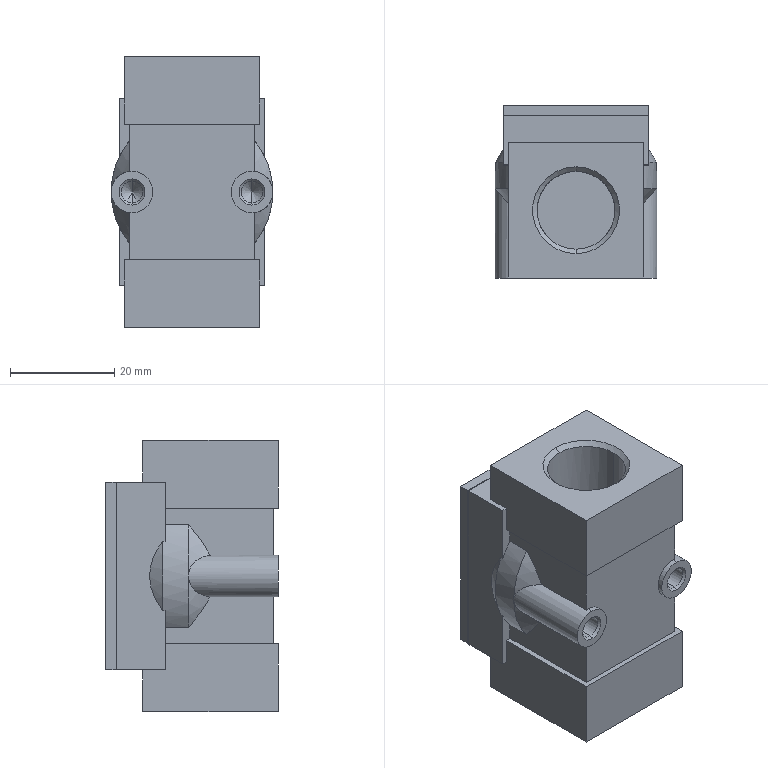Part | STEP file | _2W050-10 - Valve Body_3 | 1 solid | 67 faces | box 31 x 33.1 x 52 mm | volume 37605 mm3 | plane 35 | cone 18 | cylinder 14 | commonest cylinder face diameters 4.134 x4 8 x4 14.95 x4 31 x2